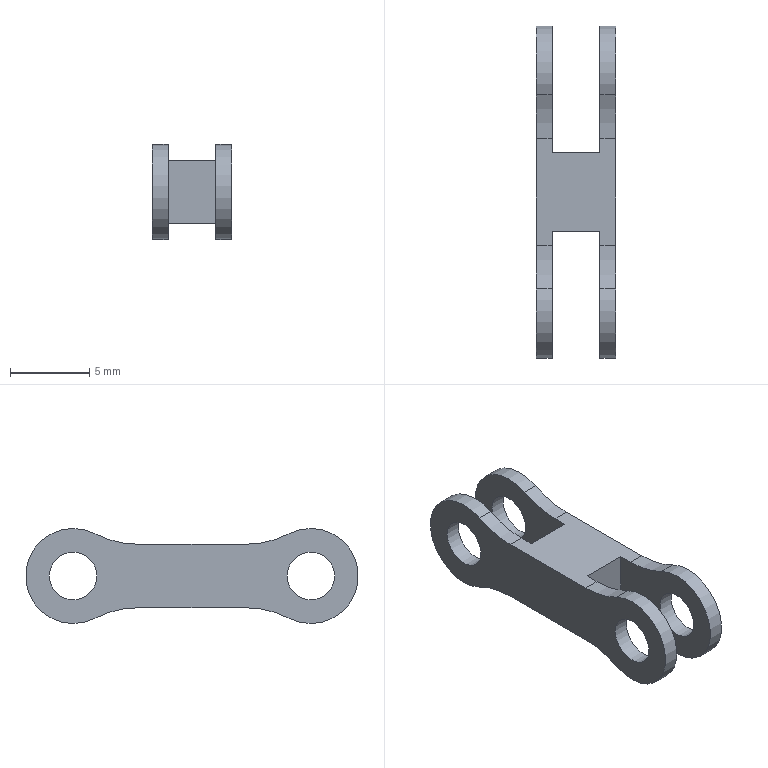Part | STEP file | 2-20 | 1 solid | 26 faces | box 5 x 21 x 6 mm | volume 222.849 mm3 | cylinder 16 | plane 10 | commonest cylinder face diameters 12 x8 3 x4 6 x4